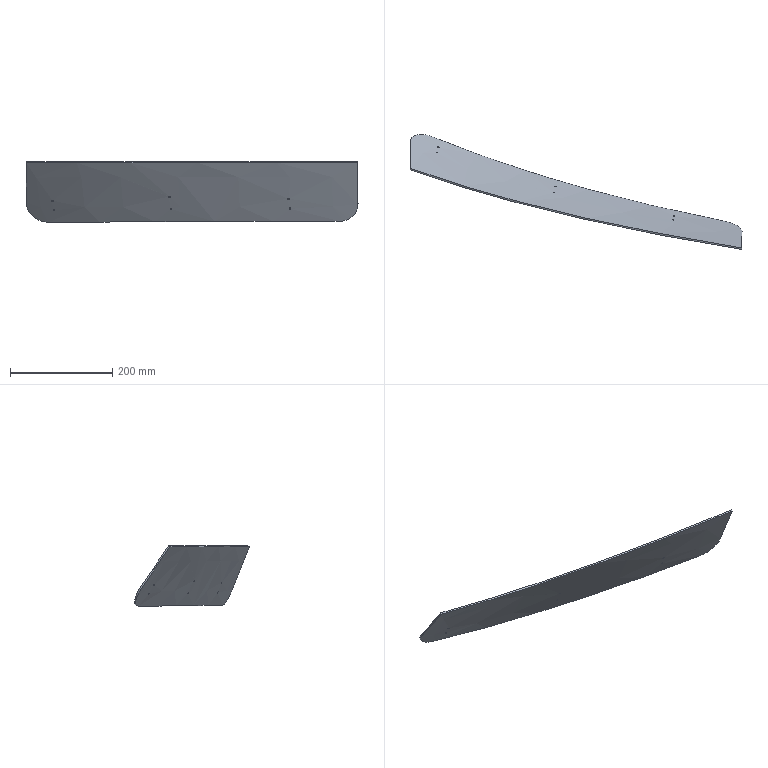Part | NX | features NG well(right door) 2 | 1 solid | 14 faces | box 650.058 x 224.899 x 118.542 mm | volume 273086 mm3 | spline 6 | cylinder 6 | plane 2 | commonest cylinder face diameters 3.175 x6